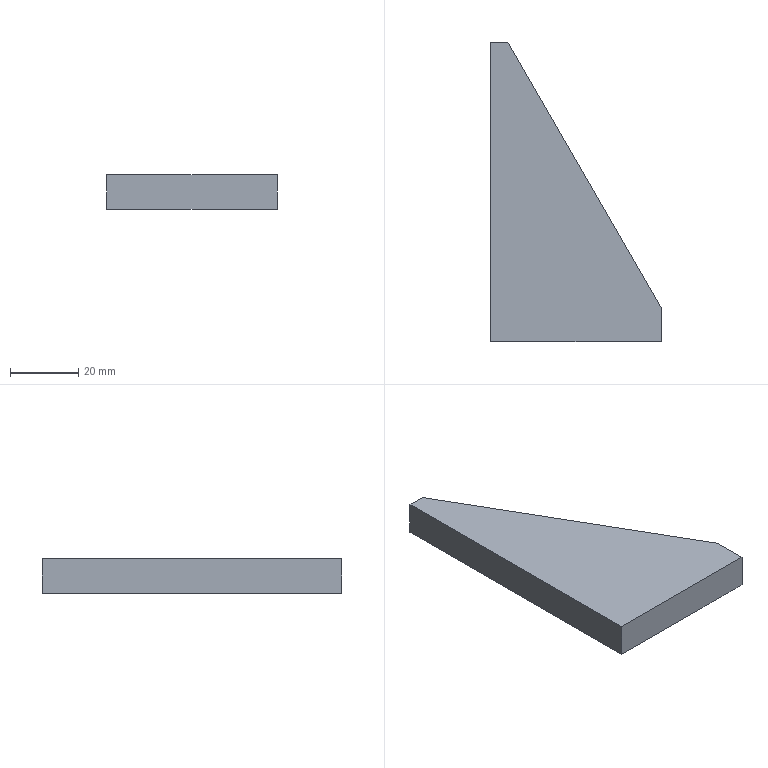Part | STEP file | X77-04103 | 1 solid | 7 faces | box 50 x 87.942 x 10 mm | volume 26434 mm3 | plane 7
STEP:
#1=CARTESIAN_POINT('',(6.108,85.365,0.));
#2=VERTEX_POINT('',#1);
#3=CARTESIAN_POINT('',(1.108,85.365,0.));
#4=VERTEX_POINT('',#3);
#5=CARTESIAN_POINT('',(1.108,85.365,0.));
#6=DIRECTION('',(-1.,0.,0.));
#7=VECTOR('',#6,1000.);
#8=LINE('',#5,#7);
#9=EDGE_CURVE('',#2,#4,#8,.T.);
#10=ORIENTED_EDGE('',*,*,#9,.T.);
#11=CARTESIAN_POINT('',(1.108,85.365,10.));
#12=VERTEX_POINT('',#11);
#13=CARTESIAN_POINT('',(1.108,85.365,10.));
#14=DIRECTION('',(0.,0.,-1.));
#15=VECTOR('',#14,1000.);
#16=LINE('',#13,#15);
#17=EDGE_CURVE('',#12,#4,#16,.T.);
#18=ORIENTED_EDGE('',*,*,#17,.F.);
#19=CARTESIAN_POINT('',(6.108,85.365,10.));
#20=VERTEX_POINT('',#19);
#21=CARTESIAN_POINT('',(1.108,85.365,10.));
#22=DIRECTION('',(-1.,0.,0.));
#23=VECTOR('',#22,1000.);
#24=LINE('',#21,#23);
#25=EDGE_CURVE('',#20,#12,#24,.T.);
#26=ORIENTED_EDGE('',*,*,#25,.F.);
#27=CARTESIAN_POINT('',(6.108,85.365,10.));
#28=DIRECTION('',(0.,0.,-1.));
#29=VECTOR('',#28,1000.);
#30=LINE('',#27,#29);
#31=EDGE_CURVE('',#20,#2,#30,.T.);
#32=ORIENTED_EDGE('',*,*,#31,.T.);
#33=EDGE_LOOP('',(#10,#18,#26,#32));
#34=FACE_OUTER_BOUND('',#33,.T.);
#35=CARTESIAN_POINT('',(1.108,85.365,10.));
#36=DIRECTION('',(0.,-1.,0.));
#37=DIRECTION('',(0.,0.,-1.));
#38=AXIS2_PLACEMENT_3D('',#35,#36,#37);
#39=PLANE('',#38);
#40=ADVANCED_FACE('',(#34),#39,.F.);
#41=CARTESIAN_POINT('',(1.108,-2.578,0.));
#42=VERTEX_POINT('',#41);
#43=CARTESIAN_POINT('',(1.108,85.365,0.));
#44=DIRECTION('',(0.,-1.,0.));
#45=VECTOR('',#44,1000.);
#46=LINE('',#43,#45);
#47=EDGE_CURVE('',#4,#42,#46,.T.);
#48=ORIENTED_EDGE('',*,*,#47,.T.);
#49=CARTESIAN_POINT('',(1.108,-2.578,10.));
#50=VERTEX_POINT('',#49);
#51=CARTESIAN_POINT('',(1.108,-2.578,10.));
#52=DIRECTION('',(0.,0.,-1.));
#53=VECTOR('',#52,1000.);
#54=LINE('',#51,#53);
#55=EDGE_CURVE('',#50,#42,#54,.T.);
#56=ORIENTED_EDGE('',*,*,#55,.F.);
#57=CARTESIAN_POINT('',(1.108,85.365,10.));
#58=DIRECTION('',(0.,-1.,0.));
#59=VECTOR('',#58,1000.);
#60=LINE('',#57,#59);
#61=EDGE_CURVE('',#12,#50,#60,.T.);
#62=ORIENTED_EDGE('',*,*,#61,.F.);
#63=ORIENTED_EDGE('',*,*,#17,.T.);
#64=EDGE_LOOP('',(#48,#56,#62,#63));
#65=FACE_OUTER_BOUND('',#64,.T.);
#66=CARTESIAN_POINT('',(1.108,85.365,10.));
#67=DIRECTION('',(1.,0.,0.));
#68=DIRECTION('',(0.,1.,0.));
#69=AXIS2_PLACEMENT_3D('',#66,#67,#68);
#70=PLANE('',#69);
#71=ADVANCED_FACE('',(#65),#70,.F.);
#72=CARTESIAN_POINT('',(51.108,-2.578,0.));
#73=VERTEX_POINT('',#72);
#74=CARTESIAN_POINT('',(1.108,-2.578,0.));
#75=DIRECTION('',(1.,0.,0.));
#76=VECTOR('',#75,1000.);
#77=LINE('',#74,#76);
#78=EDGE_CURVE('',#42,#73,#77,.T.);
#79=ORIENTED_EDGE('',*,*,#78,.T.);
#80=CARTESIAN_POINT('',(51.108,-2.578,10.));
#81=VERTEX_POINT('',#80);
#82=CARTESIAN_POINT('',(51.108,-2.578,10.));
#83=DIRECTION('',(0.,0.,-1.));
#84=VECTOR('',#83,1000.);
#85=LINE('',#82,#84);
#86=EDGE_CURVE('',#81,#73,#85,.T.);
#87=ORIENTED_EDGE('',*,*,#86,.F.);
#88=CARTESIAN_POINT('',(1.108,-2.578,10.));
#89=DIRECTION('',(1.,0.,0.));
#90=VECTOR('',#89,1000.);
#91=LINE('',#88,#90);
#92=EDGE_CURVE('',#50,#81,#91,.T.);
#93=ORIENTED_EDGE('',*,*,#92,.F.);
#94=ORIENTED_EDGE('',*,*,#55,.T.);
#95=EDGE_LOOP('',(#79,#87,#93,#94));
#96=FACE_OUTER_BOUND('',#95,.T.);
#97=CARTESIAN_POINT('',(1.108,-2.578,10.));
#98=DIRECTION('',(0.,1.,0.));
#99=DIRECTION('',(0.,0.,1.));
#100=AXIS2_PLACEMENT_3D('',#97,#98,#99);
#101=PLANE('',#100);
#102=ADVANCED_FACE('',(#96),#101,.F.);
#103=CARTESIAN_POINT('',(51.108,7.422,0.));
#104=VERTEX_POINT('',#103);
#105=CARTESIAN_POINT('',(51.108,-2.578,0.));
#106=DIRECTION('',(0.,1.,0.));
#107=VECTOR('',#106,1000.);
#108=LINE('',#105,#107);
#109=EDGE_CURVE('',#73,#104,#108,.T.);
#110=ORIENTED_EDGE('',*,*,#109,.T.);
#111=CARTESIAN_POINT('',(51.108,7.422,10.));
#112=VERTEX_POINT('',#111);
#113=CARTESIAN_POINT('',(51.108,7.422,10.));
#114=DIRECTION('',(0.,0.,-1.));
#115=VECTOR('',#114,1000.);
#116=LINE('',#113,#115);
#117=EDGE_CURVE('',#112,#104,#116,.T.);
#118=ORIENTED_EDGE('',*,*,#117,.F.);
#119=CARTESIAN_POINT('',(51.108,-2.578,10.));
#120=DIRECTION('',(0.,1.,0.));
#121=VECTOR('',#120,1000.);
#122=LINE('',#119,#121);
#123=EDGE_CURVE('',#81,#112,#122,.T.);
#124=ORIENTED_EDGE('',*,*,#123,.F.);
#125=ORIENTED_EDGE('',*,*,#86,.T.);
#126=EDGE_LOOP('',(#110,#118,#124,#125));
#127=FACE_OUTER_BOUND('',#126,.T.);
#128=CARTESIAN_POINT('',(51.108,-2.578,10.));
#129=DIRECTION('',(-1.,0.,0.));
#130=DIRECTION('',(0.,0.,1.));
#131=AXIS2_PLACEMENT_3D('',#128,#129,#130);
#132=PLANE('',#131);
#133=ADVANCED_FACE('',(#127),#132,.F.);
#134=CARTESIAN_POINT('',(51.108,7.422,0.));
#135=DIRECTION('',(-0.5,0.866,0.));
#136=VECTOR('',#135,1000.);
#137=LINE('',#134,#136);
#138=EDGE_CURVE('',#104,#2,#137,.T.);
#139=ORIENTED_EDGE('',*,*,#138,.T.);
#140=ORIENTED_EDGE('',*,*,#31,.F.);
#141=CARTESIAN_POINT('',(51.108,7.422,10.));
#142=DIRECTION('',(-0.5,0.866,0.));
#143=VECTOR('',#142,1000.);
#144=LINE('',#141,#143);
#145=EDGE_CURVE('',#112,#20,#144,.T.);
#146=ORIENTED_EDGE('',*,*,#145,.F.);
#147=ORIENTED_EDGE('',*,*,#117,.T.);
#148=EDGE_LOOP('',(#139,#140,#146,#147));
#149=FACE_OUTER_BOUND('',#148,.T.);
#150=CARTESIAN_POINT('',(51.108,7.422,10.));
#151=DIRECTION('',(-0.866,-0.5,0.));
#152=DIRECTION('',(0.5,-0.866,0.));
#153=AXIS2_PLACEMENT_3D('',#150,#151,#152);
#154=PLANE('',#153);
#155=ADVANCED_FACE('',(#149),#154,.F.);
#156=ORIENTED_EDGE('',*,*,#25,.T.);
#157=ORIENTED_EDGE('',*,*,#61,.T.);
#158=ORIENTED_EDGE('',*,*,#92,.T.);
#159=ORIENTED_EDGE('',*,*,#123,.T.);
#160=ORIENTED_EDGE('',*,*,#145,.T.);
#161=EDGE_LOOP('',(#156,#157,#158,#159,#160));
#162=FACE_OUTER_BOUND('',#161,.T.);
#163=CARTESIAN_POINT('',(51.108,85.365,10.));
#164=DIRECTION('',(0.,0.,1.));
#165=DIRECTION('',(1.,0.,0.));
#166=AXIS2_PLACEMENT_3D('',#163,#164,#165);
#167=PLANE('',#166);
#168=ADVANCED_FACE('',(#162),#167,.T.);
#169=ORIENTED_EDGE('',*,*,#9,.F.);
#170=ORIENTED_EDGE('',*,*,#138,.F.);
#171=ORIENTED_EDGE('',*,*,#109,.F.);
#172=ORIENTED_EDGE('',*,*,#78,.F.);
#173=ORIENTED_EDGE('',*,*,#47,.F.);
#174=EDGE_LOOP('',(#169,#170,#171,#172,#173));
#175=FACE_OUTER_BOUND('',#174,.T.);
#176=CARTESIAN_POINT('',(51.108,85.365,0.));
#177=DIRECTION('',(0.,0.,1.));
#178=DIRECTION('',(1.,0.,0.));
#179=AXIS2_PLACEMENT_3D('',#176,#177,#178);
#180=PLANE('',#179);
#181=ADVANCED_FACE('',(#175),#180,.F.);
#182=CLOSED_SHELL('',(#40,#71,#102,#133,#155,#168,#181));
#183=MANIFOLD_SOLID_BREP('',#182);
#184=CARTESIAN_POINT('',(0.,0.,0.));
#185=DIRECTION('',(0.,0.,1.));
#186=DIRECTION('',(1.,0.,0.));
#187=AXIS2_PLACEMENT_3D('',#184,#185,#186);
#188=(LENGTH_UNIT()NAMED_UNIT(*)SI_UNIT(.MILLI.,.METRE.));
#189=UNCERTAINTY_MEASURE_WITH_UNIT(LENGTH_MEASURE(0.00001),#188,'','');
#190=(NAMED_UNIT(*)PLANE_ANGLE_UNIT()SI_UNIT($,.RADIAN.));
#191=(NAMED_UNIT(*)SI_UNIT($,.STERADIAN.)SOLID_ANGLE_UNIT());
#192=(GEOMETRIC_REPRESENTATION_CONTEXT(3)GLOBAL_UNCERTAINTY_ASSIGNED_CONTEXT((#189))GLOBAL_UNIT_ASSIGNED_CONTEXT((#188,#190,#191))REPRESENTATION_CONTEXT('',''));
#193=ADVANCED_BREP_SHAPE_REPRESENTATION('',(#183,#187),#192);